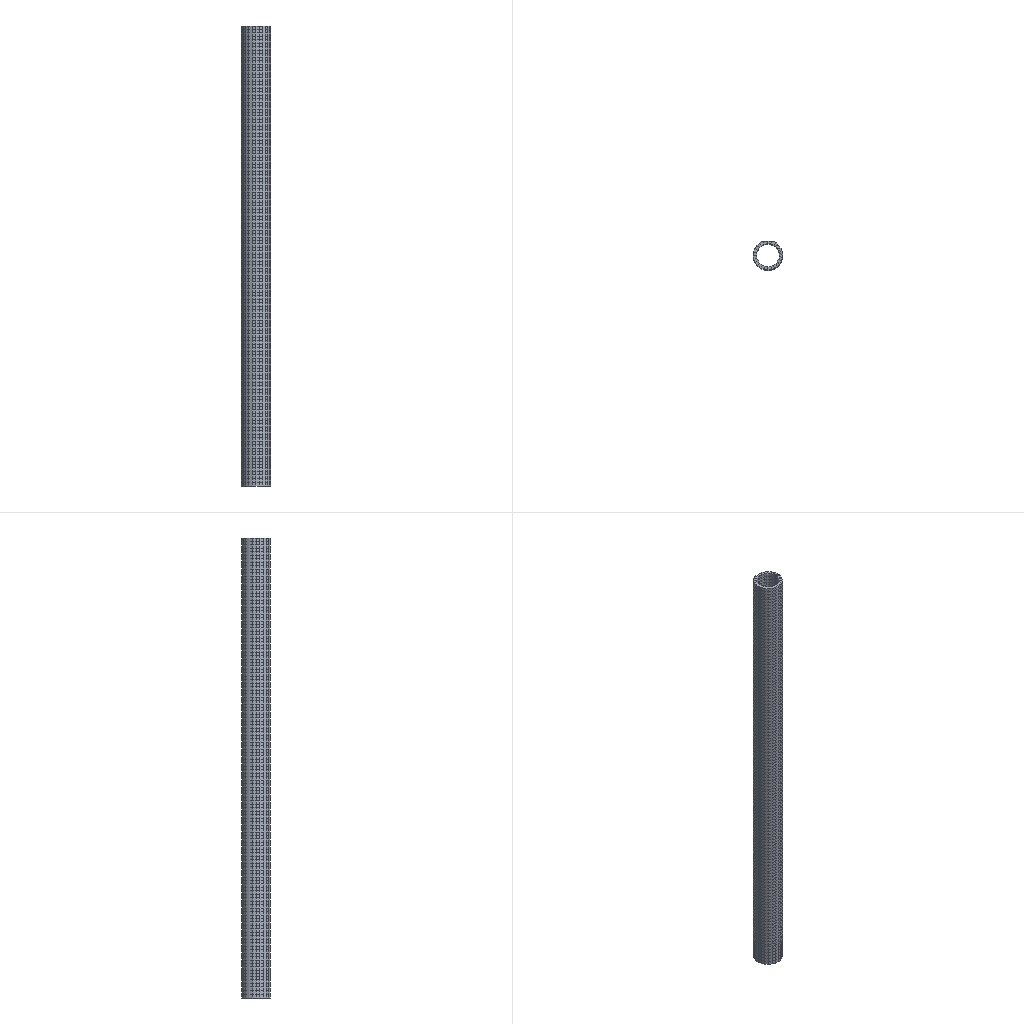Simulation study | abaqus
Set-up summary:
category,name,step,type,value,unit,region
solver,abaqus,,Abaqus/CAE 2024
units,mm-N-s-tonne (MPa),,inferred,E=210000 density=
analysis,Step-4,,static,time_period=10
mesh,nodes,,,6701
mesh,elements,,,3325
element_type,C3D8R,,,3325
material,Material-1,,E,210000
material,Material-1,,nu,0.3
material,Material-1,,yield,380
material,Material-1,,cte,1.3e-05
material,Material-1,,behaviors,plastic; expansion
section,Material-1,,solid section,,,Set-1
load,Load-2,Step-4,pressure,25,,Surf-6
load,Load-4,Step-4,concentrated force,"1000 [dir=(0, 1, 0)]",,Set-13
bc,BC-1,initial,fixed,"[dofs=rx,ry,rz,x,y,z n=6]",,Set-5
bc,BC-2,Step-4,displacement,-0.5 [dofs=rx],,_PickedSet34
bc,BC-2,Step-4,fixed,"[dofs=ry,rz n=2]",,_PickedSet34
constraint,coupling,,,1
Abaqus input file, long lists of numbers shortened:
*Heading
** Job name: deck Model name: Model-1-2-25
** Generated by: Abaqus/CAE 2024
*Preprint, echo=NO, model=NO, history=NO, contact=NO
**
** PARTS
**
*Part, name=Part-10
*Node
      1,           0.,          60.,         120.
      2,           0.,          50.,         120.
** (6698 more lines like these left out)
*Element, type=C3D8R
   1,    1,    2,   33,    5,   54,  301,  981,  549
   2,    5,   33,   34,   47,  549,  981,  982, 2479
** (3323 more lines like these left out)
*Nset, nset=Set-1, generate
    1,  6700,     1
*Elset, elset=Set-1, generate
    1,  3325,     1
** Section: Section-1
*Solid Section, elset=Set-1, material=Material-1
,
*End Part
**
**
** ASSEMBLY
**
*Assembly, name=Assembly
**
*Instance, name=Part-10-1, part=Part-10
*End Instance
**
*Node
      1,           0., -3.91886993e-15,        2000.
*Nset, nset=Set-5, instance=Part-10-1
  22,  23,  24,  25,  26,  30,  31,  32, 912, 913, 914, 915, 916, 917, 918, 919
 920, 921, 922, 923, 924, 925, 926, 927, 928, 929, 930, 931, 932, 960, 961, 962
** (2 more lines like these left out)
*Elset, elset=Set-5, instance=Part-10-1
 3210, 3211, 3212, 3213, 3214, 3215, 3216, 3217, 3218, 3219, 3220, 3221, 3313, 3314, 3315, 3316
 3317, 3318, 3319, 3320, 3321, 3322, 3323, 3324, 3325
*Nset, nset=Set-13
 1,
*Nset, nset=m_Set-12
 1,
*Nset, nset=s_Set-8, instance=Part-10-1
   8,   9,  10,  11,  12,  13,  14,  16, 674, 675, 676, 677, 678, 679, 680, 681
 682, 683, 684, 685, 686, 687, 688, 689, 690, 691, 692, 693, 694, 840, 841, 842
** (2 more lines like these left out)
*Elset, elset=s_Set-8, instance=Part-10-1
 1613, 1614, 1615, 1616, 1617, 1618, 1619, 1620, 1621, 1622, 1623, 1624, 1625, 3114, 3115, 3116
 3117, 3118, 3119, 3120, 3121, 3122, 3123, 3124, 3125
*Nset, nset=_PickedSet34, internal
 1,
*Elset, elset=_Surf-2_S3, internal, instance=Part-10-1, generate
 3126,  3221,     1
*Elset, elset=_Surf-2_S5, internal, instance=Part-10-1, generate
 3222,  3325,     1
*Elset, elset=_Surf-2_S4, internal, instance=Part-10-1, generate
    1,  1625,     1
*Elset, elset=_Surf-2_S6, internal, instance=Part-10-1, generate
 1626,  3125,     1
*Surface, type=ELEMENT, name=Surf-2
_Surf-2_S3, S3
_Surf-2_S5, S5
_Surf-2_S4, S4
_Surf-2_S6, S6
*Elset, elset=_Surf-5_S5, internal, instance=Part-10-1
 3163, 3164, 3165, 3166, 3167, 3168, 3169, 3170, 3171, 3172, 3173, 3175, 3176, 3177, 3178, 3179
 3180, 3181, 3182, 3183, 3184, 3185, 3187, 3188, 3189, 3190, 3191, 3192, 3193, 3194, 3195, 3196
** (2 more lines like these left out)
*Elset, elset=_Surf-5_S3, internal, instance=Part-10-1
 3262, 3263, 3264, 3265, 3266, 3267, 3268, 3269, 3270, 3271, 3272, 3273, 3275, 3276, 3277, 3278
 3279, 3280, 3281, 3282, 3283, 3284, 3285, 3286, 3288, 3289, 3290, 3291, 3292, 3293, 3294, 3295
** (2 more lines like these left out)
*Elset, elset=_Surf-5_S4, internal, instance=Part-10-1
 1627, 1628, 1629, 1630, 1631, 1632, 1633, 1634, 1635, 1636, 1637, 1639, 1640, 1641, 1642, 1643
 1644, 1645, 1646, 1647, 1648, 1649, 1651, 1652, 1653, 1654, 1655, 1656, 1657, 1658, 1659, 1660
** (84 more lines like these left out)
*Elset, elset=_Surf-5_S6, internal, instance=Part-10-1
    2,    3,    4,    5,    6,    7,    8,    9,   10,   11,   12,   13,   15,   16,   17,   18
   19,   20,   21,   22,   23,   24,   25,   26,   28,   29,   30,   31,   32,   33,   34,   35
** (92 more lines like these left out)
*Surface, type=ELEMENT, name=Surf-5
_Surf-5_S5, S5
_Surf-5_S3, S3
_Surf-5_S4, S4
_Surf-5_S6, S6
*Elset, elset=_Surf-6_S3, internal, instance=Part-10-1, generate
 3222,  3325,     1
*Elset, elset=_Surf-6_S5, internal, instance=Part-10-1, generate
 3126,  3221,     1
*Elset, elset=_Surf-6_S4, internal, instance=Part-10-1, generate
 1626,  3125,     1
*Elset, elset=_Surf-6_S6, internal, instance=Part-10-1, generate
    1,  1625,     1
*Surface, type=ELEMENT, name=Surf-6
_Surf-6_S3, S3
_Surf-6_S5, S5
_Surf-6_S4, S4
_Surf-6_S6, S6
*Elset, elset=_m_Surf-3_S2, internal, instance=Part-10-1
 1613, 1614, 1615, 1616, 1617, 1618, 1619, 1620, 1621, 1622, 1623, 1624, 1625, 3114, 3115, 3116
 3117, 3118, 3119, 3120, 3121, 3122, 3123, 3124, 3125
*Surface, type=ELEMENT, name=m_Surf-3
_m_Surf-3_S2, S2
*Elset, elset=_s_Surf-4_S2, internal, instance=Part-10-1
 1613, 1614, 1615, 1616, 1617, 1618, 1619, 1620, 1621, 1622, 1623, 1624, 1625, 3114, 3115, 3116
 3117, 3118, 3119, 3120, 3121, 3122, 3123, 3124, 3125
*Surface, type=ELEMENT, name=s_Surf-4
_s_Surf-4_S2, S2
** Constraint: Constraint-3
*Coupling, constraint name=Constraint-3, ref node=m_Set-12, surface=s_Surf-4
*Kinematic
*End Assembly
**
** MATERIALS
**
*Material, name=Material-1
*Elastic
210000., 0.3
*Expansion
 1.3e-05,
*Plastic
380.,  0.
600., 0.2
**
** BOUNDARY CONDITIONS
**
** Name: BC-1 Type: Displacement/Rotation
*Boundary
Set-5, 1, 1
Set-5, 2, 2
Set-5, 3, 3
Set-5, 4, 4
Set-5, 5, 5
Set-5, 6, 6
** ----------------------------------------------------------------
**
** STEP: Step-4
**
*Step, name=Step-4, nlgeom=NO, inc=1000
*Static
1., 10., 0.0001, 1.
**
** BOUNDARY CONDITIONS
**
** Name: BC-2 Type: Displacement/Rotation
*Boundary
_PickedSet34, 4, 4, -0.5
_PickedSet34, 5, 5
_PickedSet34, 6, 6
**
** LOADS
**
** Name: Load-2   Type: Pressure
*Dsload
Surf-6, P, 25.
** Name: Load-4   Type: Concentrated force
*Cload
Set-13, 2, 1000.
**
** OUTPUT REQUESTS
**
*Restart, write, frequency=0
**
** FIELD OUTPUT: F-Output-2
**
*Output, field
*Node Output
CF, RF, RM, RT, TF, U, UR, UT
V, VF, VR, VT
*Element Output, directions=YES
ALPHA, ALPHAN, BF, CENTMAG, CENTRIFMAG, CORIOMAG, CS11, CTSHR, E, EE, EEQUT, ER, ESF1, GRAV, HP, IE
LE, LODE, MISES, MISESMAX, MISESONLY, NE, NFORC, NFORCSO, P, PE, PEEQ, PEEQMAX, PEEQT, PEMAG, PEQC, PRESSONLY
PS, ROTAMAG, S, SALPHA, SE, SEE, SEP, SEPE, SEQUT, SF, SPE, SQEQ, SSAVG, TE, TEEQ, TEVOL
THE, TRIAX, TRNOR, TRSHR, TSHR, VE, VEEQ, VS, YIELDPOT
**
** HISTORY OUTPUT: H-Output-2
**
*Output, history
*Element Output
IRA1, IRA2, IRA3, IRAR1, IRAR2, IRAR3, IRF1, IRF2, IRF3, IRM1, IRM2, IRM3
*End Step
Results summary:
result,odb.job_status,,,JOB_STATUS_COMPLETED_SUCCESSFULLY,"consistent, unstated (Abaqus has no unit system)"
result,steps[0].procedure,Step-4,,*STATIC,"consistent, unstated (Abaqus has no unit system)"
result,steps[0].time_period,Step-4,,10,"consistent, unstated (Abaqus has no unit system)"
result,steps[0].n_frames,Step-4,,11,"consistent, unstated (Abaqus has no unit system)"
result,steps[0].last_frame.id,Step-4,,10,"consistent, unstated (Abaqus has no unit system)"
result,steps[0].last_frame.value,Step-4,,10,"consistent, unstated (Abaqus has no unit system)"
result,steps[0].last_frame.description,Step-4,,Increment     10: Step Time =    10.00,"consistent, unstated (Abaqus has no unit system)"
result,steps[0].completed,Step-4,,True,"consistent, unstated (Abaqus has no unit system)"
result,steps[0].max_U_magnitude,Step-4,,556.903,"consistent, unstated (Abaqus has no unit system)"
result,steps[0].max_S_mises,Step-4,,406.174,"consistent, unstated (Abaqus has no unit system)"
result,steps[0].RF_sum[1],Step-4,,-0.00119,"consistent, unstated (Abaqus has no unit system)"
result,steps[0].RF_sum[2],Step-4,,-1000,"consistent, unstated (Abaqus has no unit system)"
result,steps[0].RF_sum[3],Step-4,,-0.007812,"consistent, unstated (Abaqus has no unit system)"